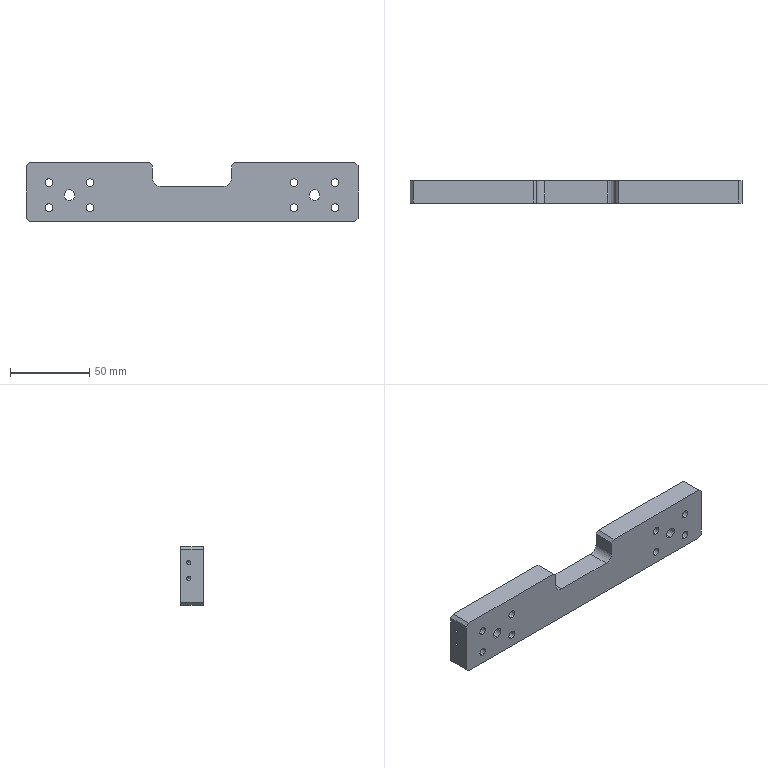Part | STEP file | PN_0021 Cylinder Plate_Default | 1 solid | 54 faces | box 210 x 14 x 37 mm | volume 94894 mm3 | cylinder 30 | plane 16 | cone 8 | commonest cylinder face diameters 5 x16 2.5 x8 6.8 x4 10 x2